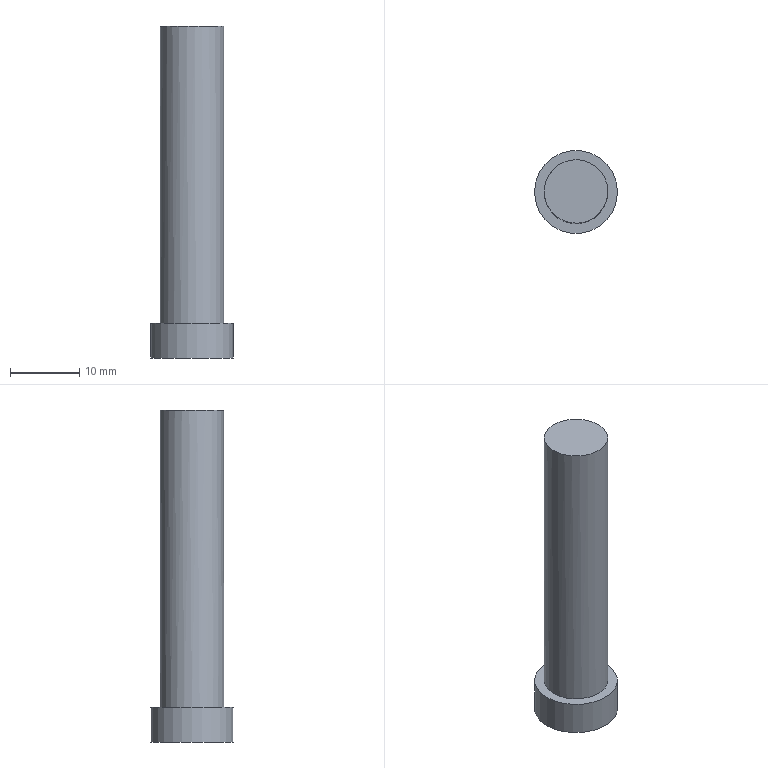Part | NX | features solid 2 | 1 solid | 5 faces | box 12 x 12 x 48 mm | volume 3424 mm3 | plane 3 | cylinder 2 | commonest cylinder face diameters 9.2 x1 12 x1
STEP:
#1=CARTESIAN_POINT('',(3326.266,-906.707,817.716));
#2=VERTEX_POINT('',#1);
#3=CARTESIAN_POINT('',(3332.266,-906.707,817.716));
#4=DIRECTION('',(0.,0.,-1.));
#5=DIRECTION('',(-1.,0.,0.));
#6=AXIS2_PLACEMENT_3D('',#3,#4,#5);
#7=CIRCLE('',#6,6.);
#8=EDGE_CURVE('',#2,#2,#7,.F.);
#9=ORIENTED_EDGE('',*,*,#8,.T.);
#10=EDGE_LOOP('',(#9));
#11=FACE_BOUND('',#10,.T.);
#12=CARTESIAN_POINT('',(3326.266,-906.707,822.716));
#13=VERTEX_POINT('',#12);
#14=CARTESIAN_POINT('',(3332.266,-906.707,822.716));
#15=DIRECTION('',(0.,0.,-1.));
#16=DIRECTION('',(-1.,0.,0.));
#17=AXIS2_PLACEMENT_3D('',#14,#15,#16);
#18=CIRCLE('',#17,6.);
#19=EDGE_CURVE('',#13,#13,#18,.F.);
#20=ORIENTED_EDGE('',*,*,#19,.F.);
#21=EDGE_LOOP('',(#20));
#22=FACE_BOUND('',#21,.T.);
#23=CARTESIAN_POINT('',(3332.266,-906.707,817.716));
#24=DIRECTION('',(0.,0.,1.));
#25=DIRECTION('',(1.,0.,0.));
#26=AXIS2_PLACEMENT_3D('',#23,#24,#25);
#27=CYLINDRICAL_SURFACE('',#26,6.);
#28=ADVANCED_FACE('',(#11,#22),#27,.T.);
#29=ORIENTED_EDGE('',*,*,#8,.F.);
#30=EDGE_LOOP('',(#29));
#31=FACE_BOUND('',#30,.T.);
#32=CARTESIAN_POINT('',(3332.266,-906.707,817.716));
#33=DIRECTION('',(0.,0.,-1.));
#34=DIRECTION('',(-1.,0.,0.));
#35=AXIS2_PLACEMENT_3D('',#32,#33,#34);
#36=PLANE('',#35);
#37=ADVANCED_FACE('',(#31),#36,.T.);
#38=CARTESIAN_POINT('',(3336.866,-906.707,822.716));
#39=VERTEX_POINT('',#38);
#40=CARTESIAN_POINT('',(3332.266,-906.707,822.716));
#41=DIRECTION('',(0.,0.,1.));
#42=DIRECTION('',(1.,0.,0.));
#43=AXIS2_PLACEMENT_3D('',#40,#41,#42);
#44=CIRCLE('',#43,4.6);
#45=EDGE_CURVE('',#39,#39,#44,.T.);
#46=ORIENTED_EDGE('',*,*,#45,.F.);
#47=EDGE_LOOP('',(#46));
#48=FACE_BOUND('',#47,.T.);
#49=ORIENTED_EDGE('',*,*,#19,.T.);
#50=EDGE_LOOP('',(#49));
#51=FACE_BOUND('',#50,.T.);
#52=CARTESIAN_POINT('',(3332.266,-906.707,822.716));
#53=DIRECTION('',(0.,0.,-1.));
#54=DIRECTION('',(-1.,0.,0.));
#55=AXIS2_PLACEMENT_3D('',#52,#53,#54);
#56=PLANE('',#55);
#57=ADVANCED_FACE('',(#48,#51),#56,.F.);
#58=CARTESIAN_POINT('',(3332.266,-902.107,865.716));
#59=VERTEX_POINT('',#58);
#60=CARTESIAN_POINT('',(3332.266,-906.707,865.716));
#61=DIRECTION('',(0.,0.,-1.));
#62=DIRECTION('',(0.,1.,0.));
#63=AXIS2_PLACEMENT_3D('',#60,#61,#62);
#64=CIRCLE('',#63,4.6);
#65=EDGE_CURVE('',#59,#59,#64,.T.);
#66=ORIENTED_EDGE('',*,*,#65,.F.);
#67=EDGE_LOOP('',(#66));
#68=FACE_BOUND('',#67,.T.);
#69=CARTESIAN_POINT('',(3353.074,-912.553,865.716));
#70=DIRECTION('',(0.,0.,-1.));
#71=DIRECTION('',(0.,1.,0.));
#72=AXIS2_PLACEMENT_3D('',#69,#70,#71);
#73=PLANE('',#72);
#74=ADVANCED_FACE('',(#68),#73,.F.);
#75=ORIENTED_EDGE('',*,*,#65,.T.);
#76=EDGE_LOOP('',(#75));
#77=FACE_BOUND('',#76,.T.);
#78=ORIENTED_EDGE('',*,*,#45,.T.);
#79=EDGE_LOOP('',(#78));
#80=FACE_BOUND('',#79,.T.);
#81=CARTESIAN_POINT('',(3332.266,-906.707,822.716));
#82=DIRECTION('',(0.,0.,1.));
#83=DIRECTION('',(1.,0.,0.));
#84=AXIS2_PLACEMENT_3D('',#81,#82,#83);
#85=CYLINDRICAL_SURFACE('',#84,4.6);
#86=ADVANCED_FACE('',(#77,#80),#85,.T.);
#87=CLOSED_SHELL('',(#28,#37,#57,#74,#86));
#88=MANIFOLD_SOLID_BREP('',#87);
#89=(LENGTH_UNIT()NAMED_UNIT(*)SI_UNIT(.MILLI.,.METRE.));
#90=UNCERTAINTY_MEASURE_WITH_UNIT(LENGTH_MEASURE(0.00001),#89,'','');
#91=(NAMED_UNIT(*)PLANE_ANGLE_UNIT()SI_UNIT($,.RADIAN.));
#92=(NAMED_UNIT(*)SI_UNIT($,.STERADIAN.)SOLID_ANGLE_UNIT());
#93=(GEOMETRIC_REPRESENTATION_CONTEXT(3)GLOBAL_UNCERTAINTY_ASSIGNED_CONTEXT((#90))GLOBAL_UNIT_ASSIGNED_CONTEXT((#89,#91,#92))REPRESENTATION_CONTEXT('',''));
#94=ADVANCED_BREP_SHAPE_REPRESENTATION('',(#88),#93);